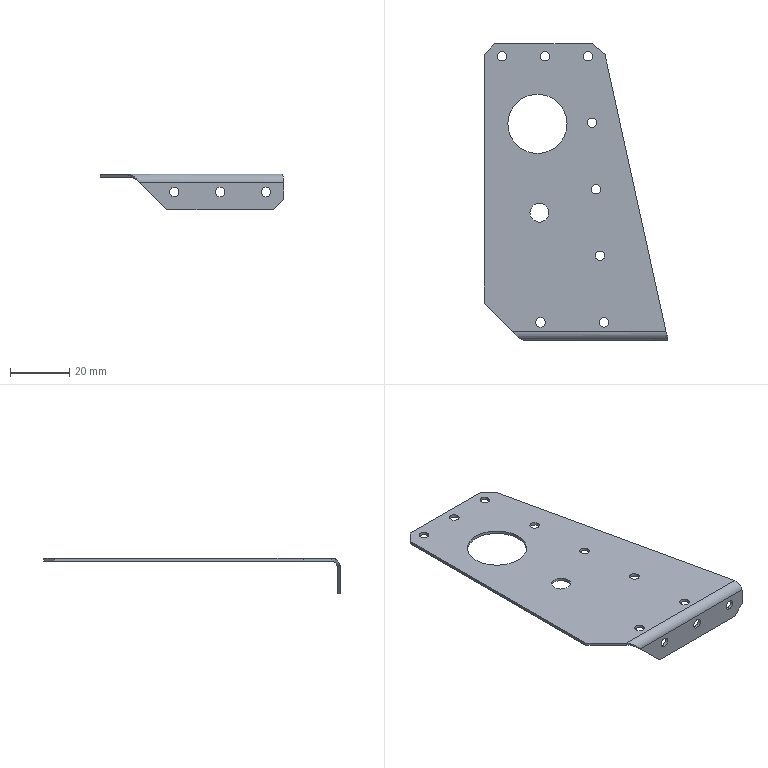Part | SolidWorks | features BaseBody 1 | 1 solid | 44 faces | box 62 x 100 x 12 mm | volume 5014 mm3 | cylinder 28 | plane 14 | spline 2 | commonest cylinder face diameters 3.2 x22 6.35 x2 20 x2 3.66 x1 5.66 x1